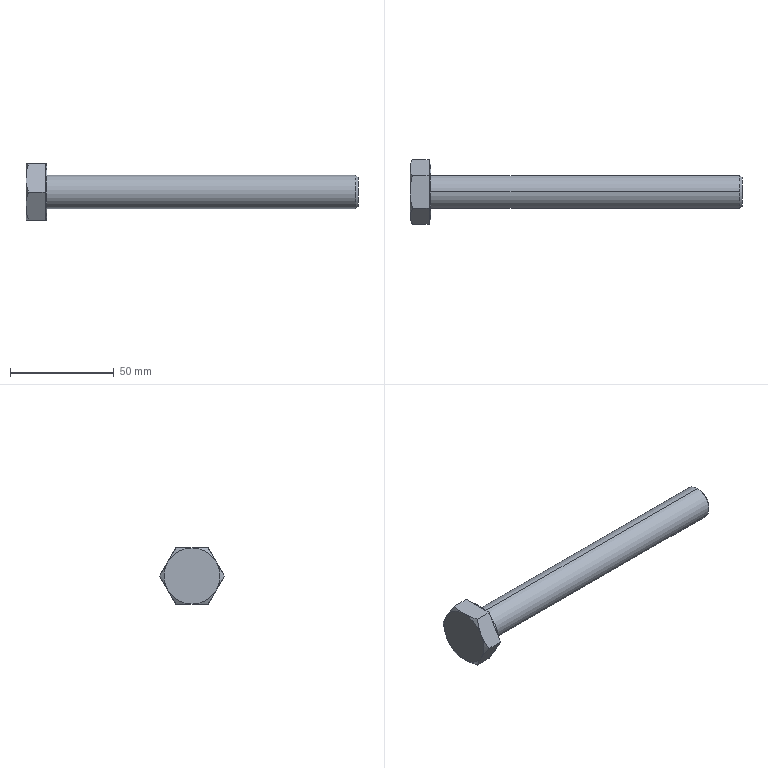Part | STEP file | hex structural bolt gradec short_iso_ISO 7412 - M16 x 150 --- 38-WN | 1 solid | 27 faces | box 160 x 31.177 x 27 mm | volume 36375 mm3 | plane 15 | cone 8 | cylinder 4 | commonest cylinder face diameters 16 x2 27 x2
STEP:
#1=CARTESIAN_POINT('',(10.,0.,-13.5));
#2=VERTEX_POINT('',#1);
#3=CARTESIAN_POINT('',(10.,0.,13.5));
#4=VERTEX_POINT('',#3);
#5=CARTESIAN_POINT('',(10.,0.,0.));
#6=DIRECTION('',(1.,0.,0.));
#7=DIRECTION('',(0.,0.,-1.));
#8=AXIS2_PLACEMENT_3D('',#5,#6,#7);
#9=CIRCLE('',#8,13.5);
#10=EDGE_CURVE('',#2,#4,#9,.T.);
#11=ORIENTED_EDGE('',*,*,#10,.F.);
#12=CARTESIAN_POINT('',(9.2,0.,-13.5));
#13=VERTEX_POINT('',#12);
#14=CARTESIAN_POINT('',(0.,0.,-13.5));
#15=DIRECTION('',(-1.,0.,0.));
#16=VECTOR('',#15,1000.);
#17=LINE('',#14,#16);
#18=EDGE_CURVE('',#2,#13,#17,.T.);
#19=ORIENTED_EDGE('',*,*,#18,.T.);
#20=CARTESIAN_POINT('',(9.2,11.691,-6.75));
#21=VERTEX_POINT('',#20);
#22=CARTESIAN_POINT('',(9.2,0.,0.));
#23=DIRECTION('',(-1.,0.,0.));
#24=DIRECTION('',(0.,0.,1.));
#25=AXIS2_PLACEMENT_3D('',#22,#23,#24);
#26=CIRCLE('',#25,13.5);
#27=EDGE_CURVE('',#21,#13,#26,.T.);
#28=ORIENTED_EDGE('',*,*,#27,.F.);
#29=CARTESIAN_POINT('',(9.2,11.691,6.75));
#30=VERTEX_POINT('',#29);
#31=CARTESIAN_POINT('',(9.2,0.,0.));
#32=DIRECTION('',(-1.,0.,0.));
#33=DIRECTION('',(0.,0.,1.));
#34=AXIS2_PLACEMENT_3D('',#31,#32,#33);
#35=CIRCLE('',#34,13.5);
#36=EDGE_CURVE('',#30,#21,#35,.T.);
#37=ORIENTED_EDGE('',*,*,#36,.F.);
#38=CARTESIAN_POINT('',(9.2,0.,13.5));
#39=VERTEX_POINT('',#38);
#40=CARTESIAN_POINT('',(9.2,0.,0.));
#41=DIRECTION('',(-1.,0.,0.));
#42=DIRECTION('',(0.,0.,1.));
#43=AXIS2_PLACEMENT_3D('',#40,#41,#42);
#44=CIRCLE('',#43,13.5);
#45=EDGE_CURVE('',#39,#30,#44,.T.);
#46=ORIENTED_EDGE('',*,*,#45,.F.);
#47=CARTESIAN_POINT('',(0.,0.,13.5));
#48=DIRECTION('',(-1.,0.,0.));
#49=VECTOR('',#48,1000.);
#50=LINE('',#47,#49);
#51=EDGE_CURVE('',#4,#39,#50,.T.);
#52=ORIENTED_EDGE('',*,*,#51,.F.);
#53=EDGE_LOOP('',(#11,#19,#28,#37,#46,#52));
#54=FACE_OUTER_BOUND('',#53,.T.);
#55=CARTESIAN_POINT('',(0.,0.,0.));
#56=DIRECTION('',(-1.,0.,0.));
#57=DIRECTION('',(0.,0.,1.));
#58=AXIS2_PLACEMENT_3D('',#55,#56,#57);
#59=CYLINDRICAL_SURFACE('',#58,13.5);
#60=ADVANCED_FACE('',(#54),#59,.T.);
#61=CARTESIAN_POINT('',(160.,0.,6.899));
#62=VERTEX_POINT('',#61);
#63=CARTESIAN_POINT('',(160.,0.,-6.899));
#64=VERTEX_POINT('',#63);
#65=CARTESIAN_POINT('',(160.,0.,0.));
#66=DIRECTION('',(-1.,0.,0.));
#67=DIRECTION('',(0.,0.,1.));
#68=AXIS2_PLACEMENT_3D('',#65,#66,#67);
#69=CIRCLE('',#68,6.899);
#70=EDGE_CURVE('',#62,#64,#69,.T.);
#71=ORIENTED_EDGE('',*,*,#70,.T.);
#72=CARTESIAN_POINT('',(158.898,0.,-8.));
#73=VERTEX_POINT('',#72);
#74=CARTESIAN_POINT('',(160.,0.,-6.899));
#75=DIRECTION('',(-0.7071,0.,-0.7071));
#76=VECTOR('',#75,1000.);
#77=LINE('',#74,#76);
#78=EDGE_CURVE('',#64,#73,#77,.T.);
#79=ORIENTED_EDGE('',*,*,#78,.T.);
#80=CARTESIAN_POINT('',(158.898,0.,8.));
#81=VERTEX_POINT('',#80);
#82=CARTESIAN_POINT('',(158.898,0.,0.));
#83=DIRECTION('',(-1.,0.,0.));
#84=DIRECTION('',(0.,0.,1.));
#85=AXIS2_PLACEMENT_3D('',#82,#83,#84);
#86=CIRCLE('',#85,8.);
#87=EDGE_CURVE('',#81,#73,#86,.T.);
#88=ORIENTED_EDGE('',*,*,#87,.F.);
#89=CARTESIAN_POINT('',(160.,0.,6.899));
#90=DIRECTION('',(-0.7071,0.,0.7071));
#91=VECTOR('',#90,1000.);
#92=LINE('',#89,#91);
#93=EDGE_CURVE('',#62,#81,#92,.T.);
#94=ORIENTED_EDGE('',*,*,#93,.F.);
#95=EDGE_LOOP('',(#71,#79,#88,#94));
#96=FACE_OUTER_BOUND('',#95,.T.);
#97=CARTESIAN_POINT('',(160.,0.,0.));
#98=DIRECTION('',(-1.,0.,0.));
#99=DIRECTION('',(0.,0.,1.));
#100=AXIS2_PLACEMENT_3D('',#97,#98,#99);
#101=CONICAL_SURFACE('',#100,6.899,0.7854);
#102=ADVANCED_FACE('',(#96),#101,.T.);
#103=ORIENTED_EDGE('',*,*,#87,.T.);
#104=CARTESIAN_POINT('',(10.,0.,-8.));
#105=VERTEX_POINT('',#104);
#106=CARTESIAN_POINT('',(0.,0.,-8.));
#107=DIRECTION('',(-1.,0.,0.));
#108=VECTOR('',#107,1000.);
#109=LINE('',#106,#108);
#110=EDGE_CURVE('',#73,#105,#109,.T.);
#111=ORIENTED_EDGE('',*,*,#110,.T.);
#112=CARTESIAN_POINT('',(10.,0.,8.));
#113=VERTEX_POINT('',#112);
#114=CARTESIAN_POINT('',(10.,0.,0.));
#115=DIRECTION('',(-1.,0.,0.));
#116=DIRECTION('',(0.,0.,-1.));
#117=AXIS2_PLACEMENT_3D('',#114,#115,#116);
#118=CIRCLE('',#117,8.);
#119=EDGE_CURVE('',#113,#105,#118,.T.);
#120=ORIENTED_EDGE('',*,*,#119,.F.);
#121=CARTESIAN_POINT('',(0.,0.,8.));
#122=DIRECTION('',(-1.,0.,0.));
#123=VECTOR('',#122,1000.);
#124=LINE('',#121,#123);
#125=EDGE_CURVE('',#81,#113,#124,.T.);
#126=ORIENTED_EDGE('',*,*,#125,.F.);
#127=EDGE_LOOP('',(#103,#111,#120,#126));
#128=FACE_OUTER_BOUND('',#127,.T.);
#129=CARTESIAN_POINT('',(0.,0.,0.));
#130=DIRECTION('',(-1.,0.,0.));
#131=DIRECTION('',(0.,0.,1.));
#132=AXIS2_PLACEMENT_3D('',#129,#130,#131);
#133=CYLINDRICAL_SURFACE('',#132,8.);
#134=ADVANCED_FACE('',(#128),#133,.T.);
#135=ORIENTED_EDGE('',*,*,#119,.T.);
#136=CARTESIAN_POINT('',(10.,0.,0.));
#137=DIRECTION('',(-1.,0.,0.));
#138=DIRECTION('',(0.,0.,-1.));
#139=AXIS2_PLACEMENT_3D('',#136,#137,#138);
#140=CIRCLE('',#139,8.);
#141=EDGE_CURVE('',#105,#113,#140,.T.);
#142=ORIENTED_EDGE('',*,*,#141,.T.);
#143=EDGE_LOOP('',(#135,#142));
#144=FACE_BOUND('',#143,.T.);
#145=CARTESIAN_POINT('',(10.,0.,0.));
#146=DIRECTION('',(1.,0.,0.));
#147=DIRECTION('',(0.,0.,-1.));
#148=AXIS2_PLACEMENT_3D('',#145,#146,#147);
#149=CIRCLE('',#148,13.5);
#150=EDGE_CURVE('',#4,#2,#149,.T.);
#151=ORIENTED_EDGE('',*,*,#150,.T.);
#152=ORIENTED_EDGE('',*,*,#10,.T.);
#153=EDGE_LOOP('',(#151,#152));
#154=FACE_OUTER_BOUND('',#153,.T.);
#155=CARTESIAN_POINT('',(10.,15.588,0.));
#156=DIRECTION('',(1.,0.,0.));
#157=DIRECTION('',(0.,0.,-1.));
#158=AXIS2_PLACEMENT_3D('',#155,#156,#157);
#159=PLANE('',#158);
#160=ADVANCED_FACE('',(#144,#154),#159,.T.);
#161=ORIENTED_EDGE('',*,*,#110,.F.);
#162=CARTESIAN_POINT('',(158.898,0.,0.));
#163=DIRECTION('',(-1.,0.,0.));
#164=DIRECTION('',(0.,0.,1.));
#165=AXIS2_PLACEMENT_3D('',#162,#163,#164);
#166=CIRCLE('',#165,8.);
#167=EDGE_CURVE('',#73,#81,#166,.T.);
#168=ORIENTED_EDGE('',*,*,#167,.T.);
#169=ORIENTED_EDGE('',*,*,#125,.T.);
#170=ORIENTED_EDGE('',*,*,#141,.F.);
#171=EDGE_LOOP('',(#161,#168,#169,#170));
#172=FACE_OUTER_BOUND('',#171,.T.);
#173=CARTESIAN_POINT('',(0.,0.,0.));
#174=DIRECTION('',(-1.,0.,0.));
#175=DIRECTION('',(0.,0.,1.));
#176=AXIS2_PLACEMENT_3D('',#173,#174,#175);
#177=CYLINDRICAL_SURFACE('',#176,8.);
#178=ADVANCED_FACE('',(#172),#177,.T.);
#179=ORIENTED_EDGE('',*,*,#78,.F.);
#180=CARTESIAN_POINT('',(160.,0.,0.));
#181=DIRECTION('',(-1.,0.,0.));
#182=DIRECTION('',(0.,0.,1.));
#183=AXIS2_PLACEMENT_3D('',#180,#181,#182);
#184=CIRCLE('',#183,6.899);
#185=EDGE_CURVE('',#64,#62,#184,.T.);
#186=ORIENTED_EDGE('',*,*,#185,.T.);
#187=ORIENTED_EDGE('',*,*,#93,.T.);
#188=ORIENTED_EDGE('',*,*,#167,.F.);
#189=EDGE_LOOP('',(#179,#186,#187,#188));
#190=FACE_OUTER_BOUND('',#189,.T.);
#191=CARTESIAN_POINT('',(160.,0.,0.));
#192=DIRECTION('',(-1.,0.,0.));
#193=DIRECTION('',(0.,0.,1.));
#194=AXIS2_PLACEMENT_3D('',#191,#192,#193);
#195=CONICAL_SURFACE('',#194,6.899,0.7854);
#196=ADVANCED_FACE('',(#190),#195,.T.);
#197=ORIENTED_EDGE('',*,*,#70,.F.);
#198=ORIENTED_EDGE('',*,*,#185,.F.);
#199=EDGE_LOOP('',(#197,#198));
#200=FACE_OUTER_BOUND('',#199,.T.);
#201=CARTESIAN_POINT('',(160.,0.,0.));
#202=DIRECTION('',(-1.,0.,0.));
#203=DIRECTION('',(0.,0.,1.));
#204=AXIS2_PLACEMENT_3D('',#201,#202,#203);
#205=PLANE('',#204);
#206=ADVANCED_FACE('',(#200),#205,.F.);
#207=CARTESIAN_POINT('',(9.2,7.794,-13.5));
#208=VERTEX_POINT('',#207);
#209=CARTESIAN_POINT('',(9.2,7.794,-13.5));
#210=DIRECTION('',(0.,0.5,0.866));
#211=VECTOR('',#210,1000.);
#212=LINE('',#209,#211);
#213=EDGE_CURVE('',#208,#21,#212,.T.);
#214=ORIENTED_EDGE('',*,*,#213,.T.);
#215=ORIENTED_EDGE('',*,*,#27,.T.);
#216=CARTESIAN_POINT('',(9.2,7.794,-13.5));
#217=DIRECTION('',(0.,1.,0.));
#218=VECTOR('',#217,1000.);
#219=LINE('',#216,#218);
#220=EDGE_CURVE('',#13,#208,#219,.T.);
#221=ORIENTED_EDGE('',*,*,#220,.T.);
#222=EDGE_LOOP('',(#214,#215,#221));
#223=FACE_OUTER_BOUND('',#222,.T.);
#224=CARTESIAN_POINT('',(9.2,13.5,0.));
#225=DIRECTION('',(1.,0.,0.));
#226=DIRECTION('',(0.,0.,-1.));
#227=AXIS2_PLACEMENT_3D('',#224,#225,#226);
#228=PLANE('',#227);
#229=ADVANCED_FACE('',(#223),#228,.T.);
#230=CARTESIAN_POINT('',(9.2,15.588,0.));
#231=VERTEX_POINT('',#230);
#232=CARTESIAN_POINT('',(9.2,7.794,-13.5));
#233=DIRECTION('',(0.,0.5,0.866));
#234=VECTOR('',#233,1000.);
#235=LINE('',#232,#234);
#236=EDGE_CURVE('',#21,#231,#235,.T.);
#237=ORIENTED_EDGE('',*,*,#236,.T.);
#238=CARTESIAN_POINT('',(9.2,15.588,0.));
#239=DIRECTION('',(0.,-0.5,0.866));
#240=VECTOR('',#239,1000.);
#241=LINE('',#238,#240);
#242=EDGE_CURVE('',#231,#30,#241,.T.);
#243=ORIENTED_EDGE('',*,*,#242,.T.);
#244=ORIENTED_EDGE('',*,*,#36,.T.);
#245=EDGE_LOOP('',(#237,#243,#244));
#246=FACE_OUTER_BOUND('',#245,.T.);
#247=CARTESIAN_POINT('',(9.2,13.5,0.));
#248=DIRECTION('',(1.,0.,0.));
#249=DIRECTION('',(0.,0.,-1.));
#250=AXIS2_PLACEMENT_3D('',#247,#248,#249);
#251=PLANE('',#250);
#252=ADVANCED_FACE('',(#246),#251,.T.);
#253=CARTESIAN_POINT('',(9.2,7.794,13.5));
#254=VERTEX_POINT('',#253);
#255=CARTESIAN_POINT('',(9.2,15.588,0.));
#256=DIRECTION('',(0.,-0.5,0.866));
#257=VECTOR('',#256,1000.);
#258=LINE('',#255,#257);
#259=EDGE_CURVE('',#30,#254,#258,.T.);
#260=ORIENTED_EDGE('',*,*,#259,.T.);
#261=CARTESIAN_POINT('',(9.2,7.794,13.5));
#262=DIRECTION('',(0.,-1.,0.));
#263=VECTOR('',#262,1000.);
#264=LINE('',#261,#263);
#265=EDGE_CURVE('',#254,#39,#264,.T.);
#266=ORIENTED_EDGE('',*,*,#265,.T.);
#267=ORIENTED_EDGE('',*,*,#45,.T.);
#268=EDGE_LOOP('',(#260,#266,#267));
#269=FACE_OUTER_BOUND('',#268,.T.);
#270=CARTESIAN_POINT('',(9.2,13.5,0.));
#271=DIRECTION('',(1.,0.,0.));
#272=DIRECTION('',(0.,0.,-1.));
#273=AXIS2_PLACEMENT_3D('',#270,#271,#272);
#274=PLANE('',#273);
#275=ADVANCED_FACE('',(#269),#274,.T.);
#276=CARTESIAN_POINT('',(9.2,-7.794,13.5));
#277=VERTEX_POINT('',#276);
#278=CARTESIAN_POINT('',(9.2,7.794,13.5));
#279=DIRECTION('',(0.,-1.,0.));
#280=VECTOR('',#279,1000.);
#281=LINE('',#278,#280);
#282=EDGE_CURVE('',#39,#277,#281,.T.);
#283=ORIENTED_EDGE('',*,*,#282,.T.);
#284=CARTESIAN_POINT('',(9.2,-11.691,6.75));
#285=VERTEX_POINT('',#284);
#286=CARTESIAN_POINT('',(9.2,-15.588,0.));
#287=DIRECTION('',(0.,-0.5,-0.866));
#288=VECTOR('',#287,1000.);
#289=LINE('',#286,#288);
#290=EDGE_CURVE('',#277,#285,#289,.T.);
#291=ORIENTED_EDGE('',*,*,#290,.T.);
#292=CARTESIAN_POINT('',(9.2,0.,0.));
#293=DIRECTION('',(-1.,0.,0.));
#294=DIRECTION('',(0.,0.,1.));
#295=AXIS2_PLACEMENT_3D('',#292,#293,#294);
#296=CIRCLE('',#295,13.5);
#297=EDGE_CURVE('',#285,#39,#296,.T.);
#298=ORIENTED_EDGE('',*,*,#297,.T.);
#299=EDGE_LOOP('',(#283,#291,#298));
#300=FACE_OUTER_BOUND('',#299,.T.);
#301=CARTESIAN_POINT('',(9.2,13.5,0.));
#302=DIRECTION('',(1.,0.,0.));
#303=DIRECTION('',(0.,0.,-1.));
#304=AXIS2_PLACEMENT_3D('',#301,#302,#303);
#305=PLANE('',#304);
#306=ADVANCED_FACE('',(#300),#305,.T.);
#307=CARTESIAN_POINT('',(9.2,-15.588,0.));
#308=VERTEX_POINT('',#307);
#309=CARTESIAN_POINT('',(9.2,-15.588,0.));
#310=DIRECTION('',(0.,-0.5,-0.866));
#311=VECTOR('',#310,1000.);
#312=LINE('',#309,#311);
#313=EDGE_CURVE('',#285,#308,#312,.T.);
#314=ORIENTED_EDGE('',*,*,#313,.T.);
#315=CARTESIAN_POINT('',(9.2,-11.691,-6.75));
#316=VERTEX_POINT('',#315);
#317=CARTESIAN_POINT('',(9.2,-7.794,-13.5));
#318=DIRECTION('',(0.,0.5,-0.866));
#319=VECTOR('',#318,1000.);
#320=LINE('',#317,#319);
#321=EDGE_CURVE('',#308,#316,#320,.T.);
#322=ORIENTED_EDGE('',*,*,#321,.T.);
#323=CARTESIAN_POINT('',(9.2,0.,0.));
#324=DIRECTION('',(-1.,0.,0.));
#325=DIRECTION('',(0.,0.,1.));
#326=AXIS2_PLACEMENT_3D('',#323,#324,#325);
#327=CIRCLE('',#326,13.5);
#328=EDGE_CURVE('',#316,#285,#327,.T.);
#329=ORIENTED_EDGE('',*,*,#328,.T.);
#330=EDGE_LOOP('',(#314,#322,#329));
#331=FACE_OUTER_BOUND('',#330,.T.);
#332=CARTESIAN_POINT('',(9.2,13.5,0.));
#333=DIRECTION('',(1.,0.,0.));
#334=DIRECTION('',(0.,0.,-1.));
#335=AXIS2_PLACEMENT_3D('',#332,#333,#334);
#336=PLANE('',#335);
#337=ADVANCED_FACE('',(#331),#336,.T.);
#338=CARTESIAN_POINT('',(9.2,-7.794,-13.5));
#339=VERTEX_POINT('',#338);
#340=CARTESIAN_POINT('',(9.2,-7.794,-13.5));
#341=DIRECTION('',(0.,0.5,-0.866));
#342=VECTOR('',#341,1000.);
#343=LINE('',#340,#342);
#344=EDGE_CURVE('',#316,#339,#343,.T.);
#345=ORIENTED_EDGE('',*,*,#344,.T.);
#346=CARTESIAN_POINT('',(9.2,7.794,-13.5));
#347=DIRECTION('',(0.,1.,0.));
#348=VECTOR('',#347,1000.);
#349=LINE('',#346,#348);
#350=EDGE_CURVE('',#339,#13,#349,.T.);
#351=ORIENTED_EDGE('',*,*,#350,.T.);
#352=CARTESIAN_POINT('',(9.2,0.,0.));
#353=DIRECTION('',(-1.,0.,0.));
#354=DIRECTION('',(0.,0.,1.));
#355=AXIS2_PLACEMENT_3D('',#352,#353,#354);
#356=CIRCLE('',#355,13.5);
#357=EDGE_CURVE('',#13,#316,#356,.T.);
#358=ORIENTED_EDGE('',*,*,#357,.T.);
#359=EDGE_LOOP('',(#345,#351,#358));
#360=FACE_OUTER_BOUND('',#359,.T.);
#361=CARTESIAN_POINT('',(9.2,13.5,0.));
#362=DIRECTION('',(1.,0.,0.));
#363=DIRECTION('',(0.,0.,-1.));
#364=AXIS2_PLACEMENT_3D('',#361,#362,#363);
#365=PLANE('',#364);
#366=ADVANCED_FACE('',(#360),#365,.T.);
#367=ORIENTED_EDGE('',*,*,#18,.F.);
#368=ORIENTED_EDGE('',*,*,#150,.F.);
#369=ORIENTED_EDGE('',*,*,#51,.T.);
#370=ORIENTED_EDGE('',*,*,#297,.F.);
#371=ORIENTED_EDGE('',*,*,#328,.F.);
#372=ORIENTED_EDGE('',*,*,#357,.F.);
#373=EDGE_LOOP('',(#367,#368,#369,#370,#371,#372));
#374=FACE_OUTER_BOUND('',#373,.T.);
#375=CARTESIAN_POINT('',(0.,0.,0.));
#376=DIRECTION('',(-1.,0.,0.));
#377=DIRECTION('',(0.,0.,1.));
#378=AXIS2_PLACEMENT_3D('',#375,#376,#377);
#379=CYLINDRICAL_SURFACE('',#378,13.5);
#380=ADVANCED_FACE('',(#374),#379,.T.);
#381=CARTESIAN_POINT('',(0.,0.,-13.5));
#382=VERTEX_POINT('',#381);
#383=CARTESIAN_POINT('',(0.,11.691,-6.75));
#384=VERTEX_POINT('',#383);
#385=CARTESIAN_POINT('',(0.,0.,0.));
#386=DIRECTION('',(1.,0.,0.));
#387=DIRECTION('',(0.,0.,-1.));
#388=AXIS2_PLACEMENT_3D('',#385,#386,#387);
#389=CIRCLE('',#388,13.5);
#390=EDGE_CURVE('',#382,#384,#389,.T.);
#391=ORIENTED_EDGE('',*,*,#390,.F.);
#392=CARTESIAN_POINT('',(0.,-11.691,-6.75));
#393=VERTEX_POINT('',#392);
#394=CARTESIAN_POINT('',(0.,0.,0.));
#395=DIRECTION('',(1.,0.,0.));
#396=DIRECTION('',(0.,0.,-1.));
#397=AXIS2_PLACEMENT_3D('',#394,#395,#396);
#398=CIRCLE('',#397,13.5);
#399=EDGE_CURVE('',#393,#382,#398,.T.);
#400=ORIENTED_EDGE('',*,*,#399,.F.);
#401=CARTESIAN_POINT('',(0.,-11.691,6.75));
#402=VERTEX_POINT('',#401);
#403=CARTESIAN_POINT('',(0.,0.,0.));
#404=DIRECTION('',(1.,0.,0.));
#405=DIRECTION('',(0.,0.,-1.));
#406=AXIS2_PLACEMENT_3D('',#403,#404,#405);
#407=CIRCLE('',#406,13.5);
#408=EDGE_CURVE('',#402,#393,#407,.T.);
#409=ORIENTED_EDGE('',*,*,#408,.F.);
#410=CARTESIAN_POINT('',(0.,0.,13.5));
#411=VERTEX_POINT('',#410);
#412=CARTESIAN_POINT('',(0.,0.,0.));
#413=DIRECTION('',(1.,0.,0.));
#414=DIRECTION('',(0.,0.,-1.));
#415=AXIS2_PLACEMENT_3D('',#412,#413,#414);
#416=CIRCLE('',#415,13.5);
#417=EDGE_CURVE('',#411,#402,#416,.T.);
#418=ORIENTED_EDGE('',*,*,#417,.F.);
#419=CARTESIAN_POINT('',(0.,11.691,6.75));
#420=VERTEX_POINT('',#419);
#421=CARTESIAN_POINT('',(0.,0.,0.));
#422=DIRECTION('',(-1.,0.,0.));
#423=DIRECTION('',(0.,0.,1.));
#424=AXIS2_PLACEMENT_3D('',#421,#422,#423);
#425=CIRCLE('',#424,13.5);
#426=EDGE_CURVE('',#411,#420,#425,.T.);
#427=ORIENTED_EDGE('',*,*,#426,.T.);
#428=CARTESIAN_POINT('',(0.,0.,0.));
#429=DIRECTION('',(1.,0.,0.));
#430=DIRECTION('',(0.,0.,-1.));
#431=AXIS2_PLACEMENT_3D('',#428,#429,#430);
#432=CIRCLE('',#431,13.5);
#433=EDGE_CURVE('',#384,#420,#432,.T.);
#434=ORIENTED_EDGE('',*,*,#433,.F.);
#435=EDGE_LOOP('',(#391,#400,#409,#418,#427,#434));
#436=FACE_OUTER_BOUND('',#435,.T.);
#437=CARTESIAN_POINT('',(0.,15.588,0.));
#438=DIRECTION('',(1.,0.,0.));
#439=DIRECTION('',(0.,0.,-1.));
#440=AXIS2_PLACEMENT_3D('',#437,#438,#439);
#441=PLANE('',#440);
#442=ADVANCED_FACE('',(#436),#441,.F.);
#443=CARTESIAN_POINT('',(1.206,15.588,0.));
#444=VERTEX_POINT('',#443);
#445=CARTESIAN_POINT('',(0.,11.691,6.75));
#446=CARTESIAN_POINT('',(0.,12.022,6.177));
#447=CARTESIAN_POINT('',(0.0285,12.354,5.602));
#448=CARTESIAN_POINT('',(0.1388,13.011,4.463));
#449=CARTESIAN_POINT('',(0.2205,13.338,3.898));
#450=CARTESIAN_POINT('',(0.5355,14.311,2.212));
#451=CARTESIAN_POINT('',(0.8386,14.953,1.101));
#452=CARTESIAN_POINT('',(1.206,15.588,0.));
#453=B_SPLINE_CURVE_WITH_KNOTS('',3,(#445,#446,#447,#448,#449,#450,#451,#452),.UNSPECIFIED.,.F.,.F.,(4,2,2,4),(0.007887,0.009851,0.01182,0.01574),.UNSPECIFIED.);
#454=EDGE_CURVE('',#420,#444,#453,.T.);
#455=ORIENTED_EDGE('',*,*,#454,.T.);
#456=CARTESIAN_POINT('',(1.206,15.588,0.));
#457=CARTESIAN_POINT('',(0.8377,14.951,-1.104));
#458=CARTESIAN_POINT('',(0.5345,14.309,-2.216));
#459=CARTESIAN_POINT('',(0.1149,13.011,-4.464));
#460=CARTESIAN_POINT('',(0.,12.355,-5.6));
#461=CARTESIAN_POINT('',(0.,11.691,-6.75));
#462=B_SPLINE_CURVE_WITH_KNOTS('',3,(#456,#457,#458,#459,#460,#461),.UNSPECIFIED.,.F.,.F.,(4,2,4),(0.000000238,0.003943,0.007887),.UNSPECIFIED.);
#463=EDGE_CURVE('',#444,#384,#462,.T.);
#464=ORIENTED_EDGE('',*,*,#463,.T.);
#465=ORIENTED_EDGE('',*,*,#433,.T.);
#466=EDGE_LOOP('',(#455,#464,#465));
#467=FACE_OUTER_BOUND('',#466,.T.);
#468=CARTESIAN_POINT('',(0.,0.,0.));
#469=DIRECTION('',(1.,0.,0.));
#470=DIRECTION('',(0.,0.,-1.));
#471=AXIS2_PLACEMENT_3D('',#468,#469,#470);
#472=CONICAL_SURFACE('',#471,13.5,1.047);
#473=ADVANCED_FACE('',(#467),#472,.T.);
#474=CARTESIAN_POINT('',(1.206,7.794,13.5));
#475=VERTEX_POINT('',#474);
#476=CARTESIAN_POINT('',(0.,0.,13.5));
#477=CARTESIAN_POINT('',(0.,0.6597,13.5));
#478=CARTESIAN_POINT('',(0.02816,1.323,13.5));
#479=CARTESIAN_POINT('',(0.1397,2.65,13.5));
#480=CARTESIAN_POINT('',(0.2222,3.306,13.5));
#481=CARTESIAN_POINT('',(0.539,5.257,13.5));
#482=CARTESIAN_POINT('',(0.8419,6.534,13.5));
#483=CARTESIAN_POINT('',(1.206,7.794,13.5));
#484=B_SPLINE_CURVE_WITH_KNOTS('',3,(#476,#477,#478,#479,#480,#481,#482,#483),.UNSPECIFIED.,.F.,.F.,(4,2,2,4),(0.02224,0.02422,0.02619,0.03014),.UNSPECIFIED.);
#485=EDGE_CURVE('',#411,#475,#484,.T.);
#486=ORIENTED_EDGE('',*,*,#485,.T.);
#487=CARTESIAN_POINT('',(1.206,7.794,13.5));
#488=CARTESIAN_POINT('',(0.8377,8.432,12.396));
#489=CARTESIAN_POINT('',(0.5345,9.074,11.284));
#490=CARTESIAN_POINT('',(0.1149,10.372,9.036));
#491=CARTESIAN_POINT('',(0.,11.027,7.9));
#492=CARTESIAN_POINT('',(0.,11.691,6.75));
#493=B_SPLINE_CURVE_WITH_KNOTS('',3,(#487,#488,#489,#490,#491,#492),.UNSPECIFIED.,.F.,.F.,(4,2,4),(0.000000238,0.003943,0.007887),.UNSPECIFIED.);
#494=EDGE_CURVE('',#475,#420,#493,.T.);
#495=ORIENTED_EDGE('',*,*,#494,.T.);
#496=ORIENTED_EDGE('',*,*,#426,.F.);
#497=EDGE_LOOP('',(#486,#495,#496));
#498=FACE_OUTER_BOUND('',#497,.T.);
#499=CARTESIAN_POINT('',(0.,0.,0.));
#500=DIRECTION('',(1.,0.,0.));
#501=DIRECTION('',(0.,0.,-1.));
#502=AXIS2_PLACEMENT_3D('',#499,#500,#501);
#503=CONICAL_SURFACE('',#502,13.5,1.047);
#504=ADVANCED_FACE('',(#498),#503,.T.);
#505=CARTESIAN_POINT('',(1.206,-7.794,13.5));
#506=VERTEX_POINT('',#505);
#507=CARTESIAN_POINT('',(1.206,-7.794,13.5));
#508=CARTESIAN_POINT('',(0.8395,-6.525,13.5));
#509=CARTESIAN_POINT('',(0.5328,-5.228,13.5));
#510=CARTESIAN_POINT('',(0.1134,-2.627,13.5));
#511=CARTESIAN_POINT('',(0.,-1.318,13.5));
#512=CARTESIAN_POINT('',(0.,0.,13.5));
#513=B_SPLINE_CURVE_WITH_KNOTS('',3,(#507,#508,#509,#510,#511,#512),.UNSPECIFIED.,.F.,.F.,(4,2,4),(0.01435,0.0183,0.02224),.UNSPECIFIED.);
#514=EDGE_CURVE('',#506,#411,#513,.T.);
#515=ORIENTED_EDGE('',*,*,#514,.T.);
#516=ORIENTED_EDGE('',*,*,#417,.T.);
#517=CARTESIAN_POINT('',(0.,-11.691,6.75));
#518=CARTESIAN_POINT('',(0.,-11.361,7.323));
#519=CARTESIAN_POINT('',(0.0285,-11.028,7.898));
#520=CARTESIAN_POINT('',(0.1388,-10.371,9.037));
#521=CARTESIAN_POINT('',(0.2205,-10.045,9.602));
#522=CARTESIAN_POINT('',(0.5355,-9.071,11.288));
#523=CARTESIAN_POINT('',(0.8386,-8.43,12.399));
#524=CARTESIAN_POINT('',(1.206,-7.794,13.5));
#525=B_SPLINE_CURVE_WITH_KNOTS('',3,(#517,#518,#519,#520,#521,#522,#523,#524),.UNSPECIFIED.,.F.,.F.,(4,2,2,4),(0.007887,0.009851,0.01182,0.01574),.UNSPECIFIED.);
#526=EDGE_CURVE('',#402,#506,#525,.T.);
#527=ORIENTED_EDGE('',*,*,#526,.T.);
#528=EDGE_LOOP('',(#515,#516,#527));
#529=FACE_OUTER_BOUND('',#528,.T.);
#530=CARTESIAN_POINT('',(0.,0.,0.));
#531=DIRECTION('',(1.,0.,0.));
#532=DIRECTION('',(0.,0.,-1.));
#533=AXIS2_PLACEMENT_3D('',#530,#531,#532);
#534=CONICAL_SURFACE('',#533,13.5,1.047);
#535=ADVANCED_FACE('',(#529),#534,.T.);
#536=CARTESIAN_POINT('',(1.206,-15.588,0.));
#537=VERTEX_POINT('',#536);
#538=CARTESIAN_POINT('',(1.206,-15.588,0.));
#539=CARTESIAN_POINT('',(0.8377,-14.951,1.104));
#540=CARTESIAN_POINT('',(0.5345,-14.309,2.216));
#541=CARTESIAN_POINT('',(0.1149,-13.011,4.464));
#542=CARTESIAN_POINT('',(0.,-12.355,5.6));
#543=CARTESIAN_POINT('',(0.,-11.691,6.75));
#544=B_SPLINE_CURVE_WITH_KNOTS('',3,(#538,#539,#540,#541,#542,#543),.UNSPECIFIED.,.F.,.F.,(4,2,4),(0.000000238,0.003943,0.007887),.UNSPECIFIED.);
#545=EDGE_CURVE('',#537,#402,#544,.T.);
#546=ORIENTED_EDGE('',*,*,#545,.T.);
#547=ORIENTED_EDGE('',*,*,#408,.T.);
#548=CARTESIAN_POINT('',(0.,-11.691,-6.75));
#549=CARTESIAN_POINT('',(0.,-12.022,-6.177));
#550=CARTESIAN_POINT('',(0.0285,-12.354,-5.602));
#551=CARTESIAN_POINT('',(0.1388,-13.011,-4.463));
#552=CARTESIAN_POINT('',(0.2205,-13.338,-3.898));
#553=CARTESIAN_POINT('',(0.5355,-14.311,-2.212));
#554=CARTESIAN_POINT('',(0.8386,-14.953,-1.101));
#555=CARTESIAN_POINT('',(1.206,-15.588,0.));
#556=B_SPLINE_CURVE_WITH_KNOTS('',3,(#548,#549,#550,#551,#552,#553,#554,#555),.UNSPECIFIED.,.F.,.F.,(4,2,2,4),(0.007887,0.009851,0.01182,0.01574),.UNSPECIFIED.);
#557=EDGE_CURVE('',#393,#537,#556,.T.);
#558=ORIENTED_EDGE('',*,*,#557,.T.);
#559=EDGE_LOOP('',(#546,#547,#558));
#560=FACE_OUTER_BOUND('',#559,.T.);
#561=CARTESIAN_POINT('',(0.,0.,0.));
#562=DIRECTION('',(1.,0.,0.));
#563=DIRECTION('',(0.,0.,-1.));
#564=AXIS2_PLACEMENT_3D('',#561,#562,#563);
#565=CONICAL_SURFACE('',#564,13.5,1.047);
#566=ADVANCED_FACE('',(#560),#565,.T.);
#567=CARTESIAN_POINT('',(1.206,7.794,-13.5));
#568=VERTEX_POINT('',#567);
#569=CARTESIAN_POINT('',(0.,11.691,-6.75));
#570=CARTESIAN_POINT('',(0.,11.361,-7.323));
#571=CARTESIAN_POINT('',(0.0285,11.028,-7.898));
#572=CARTESIAN_POINT('',(0.1388,10.371,-9.037));
#573=CARTESIAN_POINT('',(0.2205,10.045,-9.602));
#574=CARTESIAN_POINT('',(0.5355,9.071,-11.288));
#575=CARTESIAN_POINT('',(0.8386,8.43,-12.399));
#576=CARTESIAN_POINT('',(1.206,7.794,-13.5));
#577=B_SPLINE_CURVE_WITH_KNOTS('',3,(#569,#570,#571,#572,#573,#574,#575,#576),.UNSPECIFIED.,.F.,.F.,(4,2,2,4),(0.007887,0.009851,0.01182,0.01574),.UNSPECIFIED.);
#578=EDGE_CURVE('',#384,#568,#577,.T.);
#579=ORIENTED_EDGE('',*,*,#578,.T.);
#580=CARTESIAN_POINT('',(1.206,7.794,-13.5));
#581=CARTESIAN_POINT('',(0.8419,6.534,-13.5));
#582=CARTESIAN_POINT('',(0.539,5.257,-13.5));
#583=CARTESIAN_POINT('',(0.2222,3.306,-13.5));
#584=CARTESIAN_POINT('',(0.1397,2.65,-13.5));
#585=CARTESIAN_POINT('',(0.02816,1.323,-13.5));
#586=CARTESIAN_POINT('',(0.,0.6597,-13.5));
#587=CARTESIAN_POINT('',(0.,0.,-13.5));
#588=B_SPLINE_CURVE_WITH_KNOTS('',3,(#580,#581,#582,#583,#584,#585,#586,#587),.UNSPECIFIED.,.F.,.F.,(4,2,2,4),(0.03601,0.03996,0.04194,0.04391),.UNSPECIFIED.);
#589=EDGE_CURVE('',#568,#382,#588,.T.);
#590=ORIENTED_EDGE('',*,*,#589,.T.);
#591=ORIENTED_EDGE('',*,*,#390,.T.);
#592=EDGE_LOOP('',(#579,#590,#591));
#593=FACE_OUTER_BOUND('',#592,.T.);
#594=CARTESIAN_POINT('',(0.,0.,0.));
#595=DIRECTION('',(1.,0.,0.));
#596=DIRECTION('',(0.,0.,-1.));
#597=AXIS2_PLACEMENT_3D('',#594,#595,#596);
#598=CONICAL_SURFACE('',#597,13.5,1.047);
#599=ADVANCED_FACE('',(#593),#598,.T.);
#600=CARTESIAN_POINT('',(1.206,-7.794,-13.5));
#601=VERTEX_POINT('',#600);
#602=CARTESIAN_POINT('',(1.206,-7.794,-13.5));
#603=CARTESIAN_POINT('',(0.8377,-8.432,-12.396));
#604=CARTESIAN_POINT('',(0.5345,-9.074,-11.284));
#605=CARTESIAN_POINT('',(0.1149,-10.372,-9.036));
#606=CARTESIAN_POINT('',(0.,-11.027,-7.9));
#607=CARTESIAN_POINT('',(0.,-11.691,-6.75));
#608=B_SPLINE_CURVE_WITH_KNOTS('',3,(#602,#603,#604,#605,#606,#607),.UNSPECIFIED.,.F.,.F.,(4,2,4),(0.000000238,0.003943,0.007887),.UNSPECIFIED.);
#609=EDGE_CURVE('',#601,#393,#608,.T.);
#610=ORIENTED_EDGE('',*,*,#609,.T.);
#611=ORIENTED_EDGE('',*,*,#399,.T.);
#612=CARTESIAN_POINT('',(0.,0.,-13.5));
#613=CARTESIAN_POINT('',(0.,-1.318,-13.5));
#614=CARTESIAN_POINT('',(0.1134,-2.627,-13.5));
#615=CARTESIAN_POINT('',(0.5328,-5.228,-13.5));
#616=CARTESIAN_POINT('',(0.8395,-6.525,-13.5));
#617=CARTESIAN_POINT('',(1.206,-7.794,-13.5));
#618=B_SPLINE_CURVE_WITH_KNOTS('',3,(#612,#613,#614,#615,#616,#617),.UNSPECIFIED.,.F.,.F.,(4,2,4),(0.04391,0.04786,0.0518),.UNSPECIFIED.);
#619=EDGE_CURVE('',#382,#601,#618,.T.);
#620=ORIENTED_EDGE('',*,*,#619,.T.);
#621=EDGE_LOOP('',(#610,#611,#620));
#622=FACE_OUTER_BOUND('',#621,.T.);
#623=CARTESIAN_POINT('',(0.,0.,0.));
#624=DIRECTION('',(1.,0.,0.));
#625=DIRECTION('',(0.,0.,-1.));
#626=AXIS2_PLACEMENT_3D('',#623,#624,#625);
#627=CONICAL_SURFACE('',#626,13.5,1.047);
#628=ADVANCED_FACE('',(#622),#627,.T.);
#629=ORIENTED_EDGE('',*,*,#350,.F.);
#630=CARTESIAN_POINT('',(10.,-7.794,-13.5));
#631=DIRECTION('',(-1.,0.,0.));
#632=VECTOR('',#631,1000.);
#633=LINE('',#630,#632);
#634=EDGE_CURVE('',#339,#601,#633,.T.);
#635=ORIENTED_EDGE('',*,*,#634,.T.);
#636=ORIENTED_EDGE('',*,*,#619,.F.);
#637=ORIENTED_EDGE('',*,*,#589,.F.);
#638=CARTESIAN_POINT('',(10.,7.794,-13.5));
#639=DIRECTION('',(-1.,0.,0.));
#640=VECTOR('',#639,1000.);
#641=LINE('',#638,#640);
#642=EDGE_CURVE('',#208,#568,#641,.T.);
#643=ORIENTED_EDGE('',*,*,#642,.F.);
#644=ORIENTED_EDGE('',*,*,#220,.F.);
#645=EDGE_LOOP('',(#629,#635,#636,#637,#643,#644));
#646=FACE_OUTER_BOUND('',#645,.T.);
#647=CARTESIAN_POINT('',(10.,7.794,-13.5));
#648=DIRECTION('',(0.,0.,1.));
#649=DIRECTION('',(0.,-1.,0.));
#650=AXIS2_PLACEMENT_3D('',#647,#648,#649);
#651=PLANE('',#650);
#652=ADVANCED_FACE('',(#646),#651,.F.);
#653=ORIENTED_EDGE('',*,*,#321,.F.);
#654=CARTESIAN_POINT('',(10.,-15.588,0.));
#655=DIRECTION('',(-1.,0.,0.));
#656=VECTOR('',#655,1000.);
#657=LINE('',#654,#656);
#658=EDGE_CURVE('',#308,#537,#657,.T.);
#659=ORIENTED_EDGE('',*,*,#658,.T.);
#660=ORIENTED_EDGE('',*,*,#557,.F.);
#661=ORIENTED_EDGE('',*,*,#609,.F.);
#662=ORIENTED_EDGE('',*,*,#634,.F.);
#663=ORIENTED_EDGE('',*,*,#344,.F.);
#664=EDGE_LOOP('',(#653,#659,#660,#661,#662,#663));
#665=FACE_OUTER_BOUND('',#664,.T.);
#666=CARTESIAN_POINT('',(10.,-7.794,-13.5));
#667=DIRECTION('',(0.,0.866,0.5));
#668=DIRECTION('',(0.,-0.5,0.866));
#669=AXIS2_PLACEMENT_3D('',#666,#667,#668);
#670=PLANE('',#669);
#671=ADVANCED_FACE('',(#665),#670,.F.);
#672=ORIENTED_EDGE('',*,*,#290,.F.);
#673=CARTESIAN_POINT('',(10.,-7.794,13.5));
#674=DIRECTION('',(-1.,0.,0.));
#675=VECTOR('',#674,1000.);
#676=LINE('',#673,#675);
#677=EDGE_CURVE('',#277,#506,#676,.T.);
#678=ORIENTED_EDGE('',*,*,#677,.T.);
#679=ORIENTED_EDGE('',*,*,#526,.F.);
#680=ORIENTED_EDGE('',*,*,#545,.F.);
#681=ORIENTED_EDGE('',*,*,#658,.F.);
#682=ORIENTED_EDGE('',*,*,#313,.F.);
#683=EDGE_LOOP('',(#672,#678,#679,#680,#681,#682));
#684=FACE_OUTER_BOUND('',#683,.T.);
#685=CARTESIAN_POINT('',(10.,-15.588,0.));
#686=DIRECTION('',(0.,0.866,-0.5));
#687=DIRECTION('',(0.,0.5,0.866));
#688=AXIS2_PLACEMENT_3D('',#685,#686,#687);
#689=PLANE('',#688);
#690=ADVANCED_FACE('',(#684),#689,.F.);
#691=ORIENTED_EDGE('',*,*,#265,.F.);
#692=CARTESIAN_POINT('',(10.,7.794,13.5));
#693=DIRECTION('',(-1.,0.,0.));
#694=VECTOR('',#693,1000.);
#695=LINE('',#692,#694);
#696=EDGE_CURVE('',#254,#475,#695,.T.);
#697=ORIENTED_EDGE('',*,*,#696,.T.);
#698=ORIENTED_EDGE('',*,*,#485,.F.);
#699=ORIENTED_EDGE('',*,*,#514,.F.);
#700=ORIENTED_EDGE('',*,*,#677,.F.);
#701=ORIENTED_EDGE('',*,*,#282,.F.);
#702=EDGE_LOOP('',(#691,#697,#698,#699,#700,#701));
#703=FACE_OUTER_BOUND('',#702,.T.);
#704=CARTESIAN_POINT('',(10.,7.794,13.5));
#705=DIRECTION('',(0.,0.,-1.));
#706=DIRECTION('',(0.,1.,0.));
#707=AXIS2_PLACEMENT_3D('',#704,#705,#706);
#708=PLANE('',#707);
#709=ADVANCED_FACE('',(#703),#708,.F.);
#710=ORIENTED_EDGE('',*,*,#242,.F.);
#711=CARTESIAN_POINT('',(10.,15.588,0.));
#712=DIRECTION('',(-1.,0.,0.));
#713=VECTOR('',#712,1000.);
#714=LINE('',#711,#713);
#715=EDGE_CURVE('',#231,#444,#714,.T.);
#716=ORIENTED_EDGE('',*,*,#715,.T.);
#717=ORIENTED_EDGE('',*,*,#454,.F.);
#718=ORIENTED_EDGE('',*,*,#494,.F.);
#719=ORIENTED_EDGE('',*,*,#696,.F.);
#720=ORIENTED_EDGE('',*,*,#259,.F.);
#721=EDGE_LOOP('',(#710,#716,#717,#718,#719,#720));
#722=FACE_OUTER_BOUND('',#721,.T.);
#723=CARTESIAN_POINT('',(10.,15.588,0.));
#724=DIRECTION('',(0.,-0.866,-0.5));
#725=DIRECTION('',(0.,0.5,-0.866));
#726=AXIS2_PLACEMENT_3D('',#723,#724,#725);
#727=PLANE('',#726);
#728=ADVANCED_FACE('',(#722),#727,.F.);
#729=ORIENTED_EDGE('',*,*,#213,.F.);
#730=ORIENTED_EDGE('',*,*,#642,.T.);
#731=ORIENTED_EDGE('',*,*,#578,.F.);
#732=ORIENTED_EDGE('',*,*,#463,.F.);
#733=ORIENTED_EDGE('',*,*,#715,.F.);
#734=ORIENTED_EDGE('',*,*,#236,.F.);
#735=EDGE_LOOP('',(#729,#730,#731,#732,#733,#734));
#736=FACE_OUTER_BOUND('',#735,.T.);
#737=CARTESIAN_POINT('',(10.,7.794,-13.5));
#738=DIRECTION('',(0.,-0.866,0.5));
#739=DIRECTION('',(0.,-0.5,-0.866));
#740=AXIS2_PLACEMENT_3D('',#737,#738,#739);
#741=PLANE('',#740);
#742=ADVANCED_FACE('',(#736),#741,.F.);
#743=CLOSED_SHELL('',(#60,#102,#134,#160,#178,#196,#206,#229,#252,#275,#306,#337,#366,#380,#442,#473,#504,#535,#566,#599,#628,#652,#671,#690,#709,#728,#742));
#744=MANIFOLD_SOLID_BREP('',#743);
#745=CARTESIAN_POINT('',(0.,0.,0.));
#746=DIRECTION('',(0.,0.,1.));
#747=DIRECTION('',(1.,0.,0.));
#748=AXIS2_PLACEMENT_3D('',#745,#746,#747);
#749=(LENGTH_UNIT()NAMED_UNIT(*)SI_UNIT(.MILLI.,.METRE.));
#750=UNCERTAINTY_MEASURE_WITH_UNIT(LENGTH_MEASURE(0.00001),#749,'','');
#751=(NAMED_UNIT(*)PLANE_ANGLE_UNIT()SI_UNIT($,.RADIAN.));
#752=(NAMED_UNIT(*)SI_UNIT($,.STERADIAN.)SOLID_ANGLE_UNIT());
#753=(GEOMETRIC_REPRESENTATION_CONTEXT(3)GLOBAL_UNCERTAINTY_ASSIGNED_CONTEXT((#750))GLOBAL_UNIT_ASSIGNED_CONTEXT((#749,#751,#752))REPRESENTATION_CONTEXT('',''));
#754=ADVANCED_BREP_SHAPE_REPRESENTATION('',(#744,#748),#753);